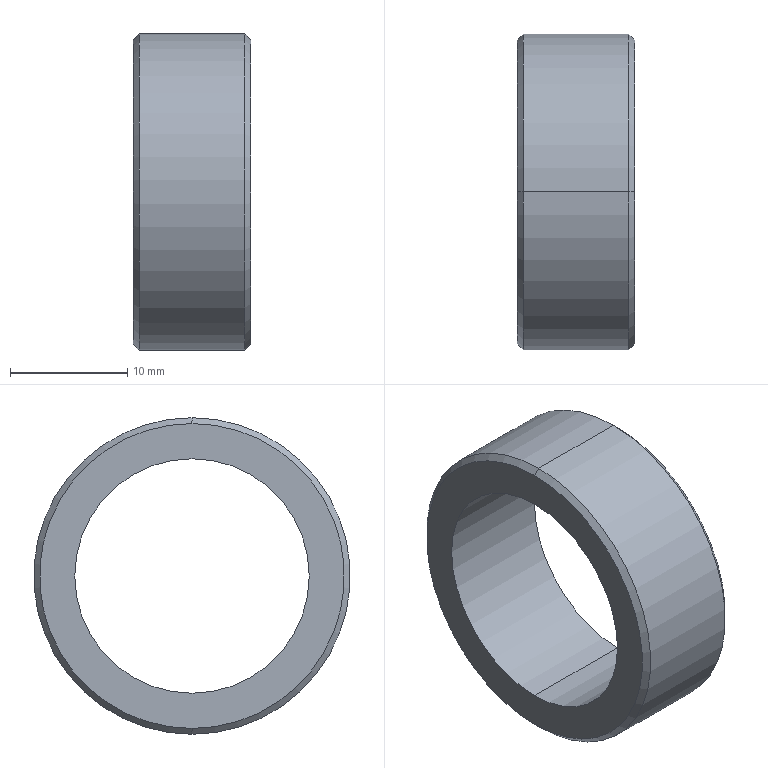Part | STEP file | CLBUS20-27-10.0 | 1 solid | 10 faces | box 10 x 27 x 27 mm | volume 2563 mm3 | cone 4 | cylinder 4 | plane 2 | commonest cylinder face diameters 20 x2 27 x2
STEP:
#1=CARTESIAN_POINT('',(10.,0.,-13.));
#2=VERTEX_POINT('',#1);
#3=CARTESIAN_POINT('',(10.,0.,13.));
#4=VERTEX_POINT('',#3);
#5=CARTESIAN_POINT('',(10.,0.,0.));
#6=DIRECTION('',(1.,0.,0.));
#7=DIRECTION('',(0.,0.,1.));
#8=AXIS2_PLACEMENT_3D('',#5,#6,#7);
#9=CIRCLE('',#8,13.);
#10=EDGE_CURVE('',#2,#4,#9,.T.);
#11=ORIENTED_EDGE('',*,*,#10,.F.);
#12=CARTESIAN_POINT('',(9.5,0.,-13.5));
#13=VERTEX_POINT('',#12);
#14=CARTESIAN_POINT('',(9.5,0.,-13.5));
#15=DIRECTION('',(-0.7071,0.,-0.7071));
#16=VECTOR('',#15,1000.);
#17=LINE('',#14,#16);
#18=EDGE_CURVE('',#2,#13,#17,.T.);
#19=ORIENTED_EDGE('',*,*,#18,.T.);
#20=CARTESIAN_POINT('',(9.5,0.,13.5));
#21=VERTEX_POINT('',#20);
#22=CARTESIAN_POINT('',(9.5,0.,0.));
#23=DIRECTION('',(-1.,0.,0.));
#24=DIRECTION('',(0.,0.,1.));
#25=AXIS2_PLACEMENT_3D('',#22,#23,#24);
#26=CIRCLE('',#25,13.5);
#27=EDGE_CURVE('',#21,#13,#26,.T.);
#28=ORIENTED_EDGE('',*,*,#27,.F.);
#29=CARTESIAN_POINT('',(9.5,0.,13.5));
#30=DIRECTION('',(-0.7071,0.,0.7071));
#31=VECTOR('',#30,1000.);
#32=LINE('',#29,#31);
#33=EDGE_CURVE('',#4,#21,#32,.T.);
#34=ORIENTED_EDGE('',*,*,#33,.F.);
#35=EDGE_LOOP('',(#11,#19,#28,#34));
#36=FACE_OUTER_BOUND('',#35,.T.);
#37=CARTESIAN_POINT('',(9.5,0.,0.));
#38=DIRECTION('',(-1.,0.,0.));
#39=DIRECTION('',(0.,0.,1.));
#40=AXIS2_PLACEMENT_3D('',#37,#38,#39);
#41=CONICAL_SURFACE('',#40,13.5,0.7854);
#42=ADVANCED_FACE('',(#36),#41,.T.);
#43=CARTESIAN_POINT('',(0.,0.,13.));
#44=VERTEX_POINT('',#43);
#45=CARTESIAN_POINT('',(0.,0.,-13.));
#46=VERTEX_POINT('',#45);
#47=CARTESIAN_POINT('',(0.,0.,0.));
#48=DIRECTION('',(-1.,0.,0.));
#49=DIRECTION('',(0.,0.,-1.));
#50=AXIS2_PLACEMENT_3D('',#47,#48,#49);
#51=CIRCLE('',#50,13.);
#52=EDGE_CURVE('',#44,#46,#51,.T.);
#53=ORIENTED_EDGE('',*,*,#52,.F.);
#54=CARTESIAN_POINT('',(0.5,0.,13.5));
#55=VERTEX_POINT('',#54);
#56=CARTESIAN_POINT('',(0.,0.,13.));
#57=DIRECTION('',(0.7071,0.,0.7071));
#58=VECTOR('',#57,1000.);
#59=LINE('',#56,#58);
#60=EDGE_CURVE('',#44,#55,#59,.T.);
#61=ORIENTED_EDGE('',*,*,#60,.T.);
#62=CARTESIAN_POINT('',(0.5,0.,-13.5));
#63=VERTEX_POINT('',#62);
#64=CARTESIAN_POINT('',(0.5,0.,0.));
#65=DIRECTION('',(1.,0.,0.));
#66=DIRECTION('',(0.,0.,-1.));
#67=AXIS2_PLACEMENT_3D('',#64,#65,#66);
#68=CIRCLE('',#67,13.5);
#69=EDGE_CURVE('',#63,#55,#68,.T.);
#70=ORIENTED_EDGE('',*,*,#69,.F.);
#71=CARTESIAN_POINT('',(0.,0.,-13.));
#72=DIRECTION('',(0.7071,0.,-0.7071));
#73=VECTOR('',#72,1000.);
#74=LINE('',#71,#73);
#75=EDGE_CURVE('',#46,#63,#74,.T.);
#76=ORIENTED_EDGE('',*,*,#75,.F.);
#77=EDGE_LOOP('',(#53,#61,#70,#76));
#78=FACE_OUTER_BOUND('',#77,.T.);
#79=CARTESIAN_POINT('',(0.,0.,0.));
#80=DIRECTION('',(1.,0.,0.));
#81=DIRECTION('',(0.,0.,-1.));
#82=AXIS2_PLACEMENT_3D('',#79,#80,#81);
#83=CONICAL_SURFACE('',#82,13.,0.7854);
#84=ADVANCED_FACE('',(#78),#83,.T.);
#85=ORIENTED_EDGE('',*,*,#27,.T.);
#86=CARTESIAN_POINT('',(0.,0.,-13.5));
#87=DIRECTION('',(-1.,0.,0.));
#88=VECTOR('',#87,1000.);
#89=LINE('',#86,#88);
#90=EDGE_CURVE('',#13,#63,#89,.T.);
#91=ORIENTED_EDGE('',*,*,#90,.T.);
#92=ORIENTED_EDGE('',*,*,#69,.T.);
#93=CARTESIAN_POINT('',(0.,0.,13.5));
#94=DIRECTION('',(-1.,0.,0.));
#95=VECTOR('',#94,1000.);
#96=LINE('',#93,#95);
#97=EDGE_CURVE('',#21,#55,#96,.T.);
#98=ORIENTED_EDGE('',*,*,#97,.F.);
#99=EDGE_LOOP('',(#85,#91,#92,#98));
#100=FACE_OUTER_BOUND('',#99,.T.);
#101=CARTESIAN_POINT('',(0.,0.,0.));
#102=DIRECTION('',(-1.,0.,0.));
#103=DIRECTION('',(0.,0.,1.));
#104=AXIS2_PLACEMENT_3D('',#101,#102,#103);
#105=CYLINDRICAL_SURFACE('',#104,13.5);
#106=ADVANCED_FACE('',(#100),#105,.T.);
#107=CARTESIAN_POINT('',(10.,0.,-10.));
#108=VERTEX_POINT('',#107);
#109=CARTESIAN_POINT('',(10.,0.,10.));
#110=VERTEX_POINT('',#109);
#111=CARTESIAN_POINT('',(10.,0.,0.));
#112=DIRECTION('',(-1.,0.,0.));
#113=DIRECTION('',(0.,0.,1.));
#114=AXIS2_PLACEMENT_3D('',#111,#112,#113);
#115=CIRCLE('',#114,10.);
#116=EDGE_CURVE('',#108,#110,#115,.T.);
#117=ORIENTED_EDGE('',*,*,#116,.F.);
#118=CARTESIAN_POINT('',(0.,0.,-10.));
#119=VERTEX_POINT('',#118);
#120=CARTESIAN_POINT('',(0.,0.,-10.));
#121=DIRECTION('',(-1.,0.,0.));
#122=VECTOR('',#121,1000.);
#123=LINE('',#120,#122);
#124=EDGE_CURVE('',#108,#119,#123,.T.);
#125=ORIENTED_EDGE('',*,*,#124,.T.);
#126=CARTESIAN_POINT('',(0.,0.,10.));
#127=VERTEX_POINT('',#126);
#128=CARTESIAN_POINT('',(0.,0.,0.));
#129=DIRECTION('',(-1.,0.,0.));
#130=DIRECTION('',(0.,0.,1.));
#131=AXIS2_PLACEMENT_3D('',#128,#129,#130);
#132=CIRCLE('',#131,10.);
#133=EDGE_CURVE('',#119,#127,#132,.T.);
#134=ORIENTED_EDGE('',*,*,#133,.T.);
#135=CARTESIAN_POINT('',(0.,0.,10.));
#136=DIRECTION('',(-1.,0.,0.));
#137=VECTOR('',#136,1000.);
#138=LINE('',#135,#137);
#139=EDGE_CURVE('',#110,#127,#138,.T.);
#140=ORIENTED_EDGE('',*,*,#139,.F.);
#141=EDGE_LOOP('',(#117,#125,#134,#140));
#142=FACE_OUTER_BOUND('',#141,.T.);
#143=CARTESIAN_POINT('',(0.,0.,0.));
#144=DIRECTION('',(-1.,0.,0.));
#145=DIRECTION('',(0.,0.,1.));
#146=AXIS2_PLACEMENT_3D('',#143,#144,#145);
#147=CYLINDRICAL_SURFACE('',#146,10.);
#148=ADVANCED_FACE('',(#142),#147,.F.);
#149=CARTESIAN_POINT('',(10.,0.,0.));
#150=DIRECTION('',(1.,0.,0.));
#151=DIRECTION('',(0.,0.,1.));
#152=AXIS2_PLACEMENT_3D('',#149,#150,#151);
#153=CIRCLE('',#152,13.);
#154=EDGE_CURVE('',#4,#2,#153,.T.);
#155=ORIENTED_EDGE('',*,*,#154,.T.);
#156=ORIENTED_EDGE('',*,*,#10,.T.);
#157=EDGE_LOOP('',(#155,#156));
#158=FACE_OUTER_BOUND('',#157,.T.);
#159=CARTESIAN_POINT('',(10.,0.,0.));
#160=DIRECTION('',(-1.,0.,0.));
#161=DIRECTION('',(0.,0.,1.));
#162=AXIS2_PLACEMENT_3D('',#159,#160,#161);
#163=CIRCLE('',#162,10.);
#164=EDGE_CURVE('',#110,#108,#163,.T.);
#165=ORIENTED_EDGE('',*,*,#164,.T.);
#166=ORIENTED_EDGE('',*,*,#116,.T.);
#167=EDGE_LOOP('',(#165,#166));
#168=FACE_BOUND('',#167,.T.);
#169=CARTESIAN_POINT('',(10.,13.5,0.));
#170=DIRECTION('',(-1.,0.,0.));
#171=DIRECTION('',(0.,0.,1.));
#172=AXIS2_PLACEMENT_3D('',#169,#170,#171);
#173=PLANE('',#172);
#174=ADVANCED_FACE('',(#158,#168),#173,.F.);
#175=ORIENTED_EDGE('',*,*,#124,.F.);
#176=ORIENTED_EDGE('',*,*,#164,.F.);
#177=ORIENTED_EDGE('',*,*,#139,.T.);
#178=CARTESIAN_POINT('',(0.,0.,0.));
#179=DIRECTION('',(-1.,0.,0.));
#180=DIRECTION('',(0.,0.,1.));
#181=AXIS2_PLACEMENT_3D('',#178,#179,#180);
#182=CIRCLE('',#181,10.);
#183=EDGE_CURVE('',#127,#119,#182,.T.);
#184=ORIENTED_EDGE('',*,*,#183,.T.);
#185=EDGE_LOOP('',(#175,#176,#177,#184));
#186=FACE_OUTER_BOUND('',#185,.T.);
#187=CARTESIAN_POINT('',(0.,0.,0.));
#188=DIRECTION('',(-1.,0.,0.));
#189=DIRECTION('',(0.,0.,1.));
#190=AXIS2_PLACEMENT_3D('',#187,#188,#189);
#191=CYLINDRICAL_SURFACE('',#190,10.);
#192=ADVANCED_FACE('',(#186),#191,.F.);
#193=CARTESIAN_POINT('',(0.,0.,0.));
#194=DIRECTION('',(-1.,0.,0.));
#195=DIRECTION('',(0.,0.,-1.));
#196=AXIS2_PLACEMENT_3D('',#193,#194,#195);
#197=CIRCLE('',#196,13.);
#198=EDGE_CURVE('',#46,#44,#197,.T.);
#199=ORIENTED_EDGE('',*,*,#198,.T.);
#200=ORIENTED_EDGE('',*,*,#52,.T.);
#201=EDGE_LOOP('',(#199,#200));
#202=FACE_OUTER_BOUND('',#201,.T.);
#203=ORIENTED_EDGE('',*,*,#183,.F.);
#204=ORIENTED_EDGE('',*,*,#133,.F.);
#205=EDGE_LOOP('',(#203,#204));
#206=FACE_BOUND('',#205,.T.);
#207=CARTESIAN_POINT('',(0.,10.,0.));
#208=DIRECTION('',(1.,0.,0.));
#209=DIRECTION('',(0.,0.,-1.));
#210=AXIS2_PLACEMENT_3D('',#207,#208,#209);
#211=PLANE('',#210);
#212=ADVANCED_FACE('',(#202,#206),#211,.F.);
#213=ORIENTED_EDGE('',*,*,#90,.F.);
#214=CARTESIAN_POINT('',(9.5,0.,0.));
#215=DIRECTION('',(-1.,0.,0.));
#216=DIRECTION('',(0.,0.,1.));
#217=AXIS2_PLACEMENT_3D('',#214,#215,#216);
#218=CIRCLE('',#217,13.5);
#219=EDGE_CURVE('',#13,#21,#218,.T.);
#220=ORIENTED_EDGE('',*,*,#219,.T.);
#221=ORIENTED_EDGE('',*,*,#97,.T.);
#222=CARTESIAN_POINT('',(0.5,0.,0.));
#223=DIRECTION('',(1.,0.,0.));
#224=DIRECTION('',(0.,0.,-1.));
#225=AXIS2_PLACEMENT_3D('',#222,#223,#224);
#226=CIRCLE('',#225,13.5);
#227=EDGE_CURVE('',#55,#63,#226,.T.);
#228=ORIENTED_EDGE('',*,*,#227,.T.);
#229=EDGE_LOOP('',(#213,#220,#221,#228));
#230=FACE_OUTER_BOUND('',#229,.T.);
#231=CARTESIAN_POINT('',(0.,0.,0.));
#232=DIRECTION('',(-1.,0.,0.));
#233=DIRECTION('',(0.,0.,1.));
#234=AXIS2_PLACEMENT_3D('',#231,#232,#233);
#235=CYLINDRICAL_SURFACE('',#234,13.5);
#236=ADVANCED_FACE('',(#230),#235,.T.);
#237=ORIENTED_EDGE('',*,*,#60,.F.);
#238=ORIENTED_EDGE('',*,*,#198,.F.);
#239=ORIENTED_EDGE('',*,*,#75,.T.);
#240=ORIENTED_EDGE('',*,*,#227,.F.);
#241=EDGE_LOOP('',(#237,#238,#239,#240));
#242=FACE_OUTER_BOUND('',#241,.T.);
#243=CARTESIAN_POINT('',(0.,0.,0.));
#244=DIRECTION('',(1.,0.,0.));
#245=DIRECTION('',(0.,0.,-1.));
#246=AXIS2_PLACEMENT_3D('',#243,#244,#245);
#247=CONICAL_SURFACE('',#246,13.,0.7854);
#248=ADVANCED_FACE('',(#242),#247,.T.);
#249=ORIENTED_EDGE('',*,*,#18,.F.);
#250=ORIENTED_EDGE('',*,*,#154,.F.);
#251=ORIENTED_EDGE('',*,*,#33,.T.);
#252=ORIENTED_EDGE('',*,*,#219,.F.);
#253=EDGE_LOOP('',(#249,#250,#251,#252));
#254=FACE_OUTER_BOUND('',#253,.T.);
#255=CARTESIAN_POINT('',(9.5,0.,0.));
#256=DIRECTION('',(-1.,0.,0.));
#257=DIRECTION('',(0.,0.,1.));
#258=AXIS2_PLACEMENT_3D('',#255,#256,#257);
#259=CONICAL_SURFACE('',#258,13.5,0.7854);
#260=ADVANCED_FACE('',(#254),#259,.T.);
#261=CLOSED_SHELL('',(#42,#84,#106,#148,#174,#192,#212,#236,#248,#260));
#262=MANIFOLD_SOLID_BREP('',#261);
#263=CARTESIAN_POINT('',(0.,0.,0.));
#264=DIRECTION('',(0.,0.,1.));
#265=DIRECTION('',(1.,0.,0.));
#266=AXIS2_PLACEMENT_3D('',#263,#264,#265);
#267=(LENGTH_UNIT()NAMED_UNIT(*)SI_UNIT(.MILLI.,.METRE.));
#268=UNCERTAINTY_MEASURE_WITH_UNIT(LENGTH_MEASURE(0.00001),#267,'','');
#269=(NAMED_UNIT(*)PLANE_ANGLE_UNIT()SI_UNIT($,.RADIAN.));
#270=(NAMED_UNIT(*)SI_UNIT($,.STERADIAN.)SOLID_ANGLE_UNIT());
#271=(GEOMETRIC_REPRESENTATION_CONTEXT(3)GLOBAL_UNCERTAINTY_ASSIGNED_CONTEXT((#268))GLOBAL_UNIT_ASSIGNED_CONTEXT((#267,#269,#270))REPRESENTATION_CONTEXT('',''));
#272=ADVANCED_BREP_SHAPE_REPRESENTATION('',(#262,#266),#271);